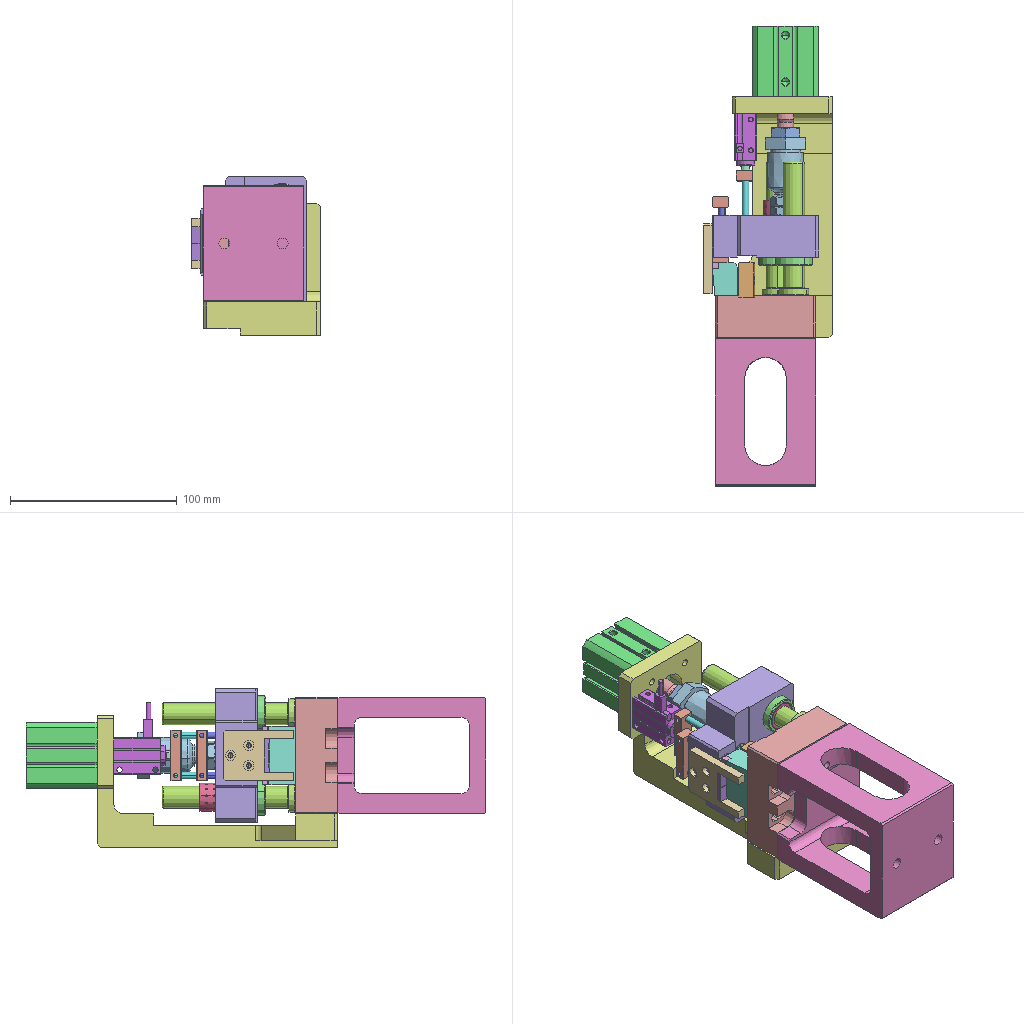Assembly | SolidWorks | 22 different items | 34 placed | box 77 x 276 x 95 mm
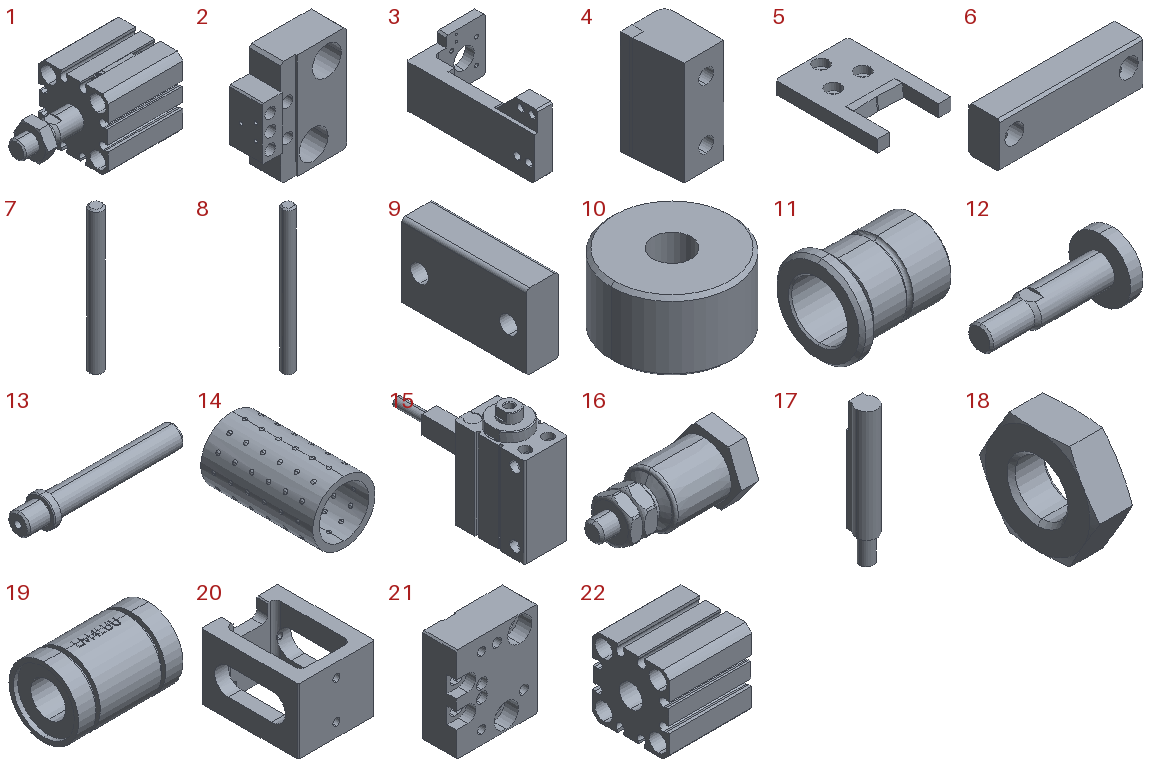Parts list (item | name | quantity | parent item | size | volume | features):
1 | (subassembly) | x1 | - | 75 x 40 x 40 mm | 54113 mm3 | features AEMSimFeature 1
2 | - | x1 | - | 64 x 25 x 80 mm | 85736 mm3 | features ICE 6, Chamfer 2, HoleWzd 2, Extrusion 1
3 | - | x1 | - | 79 x 144 x 70 mm | 147629 mm3 | features ICE 5, Chamfer 3, HoleWzd 3, Fillet 2, Extrusion 1
4 | - | x1 | - | 15 x 20 x 35 mm | 9279 mm3 | features Extrusion 1, Fillet 1, HoleWzd 1, Split 1
5 | - | x1 | - | 30 x 42 x 5 mm | 4509 mm3 | features ICE 3, Chamfer 2, Extrusion 1, Fillet 1, HoleWzd 1
6 | - | x4 | - | 30 x 6.5 x 9.5 mm | 1639 mm3 | features Chamfer 1, Extrusion 1, HoleWzd 1, ICE 1
7 | - | x2 | - | 4 x 4 x 43 mm | 530.221 mm3 | features Chamfer 1, Extrusion 1, ICE 1
8 | - | x2 | - | 4 x 4 x 50 mm | 618.186 mm3 | features Chamfer 1, Extrusion 1, ICE 1
9 | - | x1 | - | 9 x 35 x 21 mm | 5976 mm3 | features HoleWzd 2, Chamfer 1, Extrusion 1, Fillet 1
10 | - | x2 | - | 17.5 x 17.5 x 10 mm | 1853 mm3 | features Chamfer 1, Extrusion 1, ICE 1
11 | - | x2 | - | 30 x 27 x 27 mm | 5060 mm3 | features Chamfer 2, RefAxis 1, RevCut 1, Revolution 1
12 | - | x1 | in 1 | 53.75 x 25 x 25 mm | 7288 mm3 | features RefAxis 6, 3DProfileFeature 2, ICE 1, Revolution 1
13 | - | x2 | - | 93 x 18 x 18 mm | 12586 mm3 | features Chamfer 2, Fillet 1, HoleWzd 1, Revolution 1
14 | - | x2 | - | 17 x 30 x 17 mm | 2413 mm3 | features CirPattern 2, LPattern 2, RefAxis 2, Extrusion 1, ICE 1, Revolution 1
15 | - | x1 | - | 13.5 x 43.2 x 34 mm | 7865 mm3 | features BaseBody 2
16 | - | x1 | - | 54 x 27.472 x 25.615 mm | 13856 mm3 | features ICE 2, Revolution 1
17 | - | x1 | in 1 | 4 x 4.5 x 27 mm | 342.413 mm3 | features ICE 3, RefAxis 3, 3DProfileFeature 1, Extrusion 1, Revolution 1
18 | - | x1 | in 1 | 6 x 19.63 x 17 mm | 1131 mm3 | features RefAxis 3, 3DProfileFeature 1, ICE 1, Revolution 1
19 | - | x4 | - | 12 x 8 x 8 mm | 414.691 mm3 | features Emboss 1, Revolution 1
20 | - | x1 | - | 70 x 89 x 60 mm | 142318 mm3 | features HoleWzd 4, Fillet 2, ICE 2, Chamfer 1, Extrusion 1
21 | - | x1 | - | 60 x 25 x 70 mm | 85234 mm3 | features HoleWzd 7, ICE 3, Chamfer 1, Cut 1, Extrusion 1
22 | - | x1 | in 1 | 42.5 x 40 x 40 mm | 45351 mm3 | features RefAxis 18, 3DProfileFeature 6, HoleWzd 2, RevCut 2, Extrusion 1, LPattern 1
Mates (type | each side: item.copy, entity, surface, feature):
In the top assembly
Concentric | 21.1 face cylinder Cut-Extrude2 | 10.1 face cylinder Boss-Extrude1
Coincident | 21.1 face plane Cut-Extrude2 | 10.1 face plane Boss-Extrude1
Concentric | 21.1 face cylinder Cut-Extrude2 | 10.2 face cylinder Boss-Extrude1
Coincident | 21.1 face plane Cut-Extrude2 | 10.2 face plane Boss-Extrude1
Concentric | 21.1 face cylinder Cut-Extrude1 | 13.1 face cylinder Revolve1
Coincident | 21.1 face plane Boss-Extrude1 | 13.1 face plane Revolve1
Concentric | 21.1 face cylinder Cut-Extrude1 | 13.2 face cylinder Revolve1
Coincident | 21.1 face plane Boss-Extrude1 | 13.2 face plane Revolve1
Width | 21.1 face plane Cut-Extrude1 | 21.1 face plane Cut-Extrude1 | 4.1 face cylinder M6 Tapped Hole1 | 2 times
Coincident | 21.1 face plane Boss-Extrude1 | 4.1 face plane Boss-Extrude1
Coincident | 21.1 face plane Cut-Extrude3 | 9.1 face plane Boss-Extrude1
Concentric | 11.1 face cylinder Revolve1 | 14.1 face cylinder Boss-Extrude1
Coincident | 11.1 face plane Revolve1 | 14.1 face plane Boss-Extrude1
Concentric | 11.2 face cylinder Revolve1 | 14.2 face cylinder Boss-Extrude1
Concentric | 2.1 face cylinder Cut-Extrude1 | 11.2 face cylinder Revolve1
Concentric | 2.1 face cylinder Cut-Extrude1 | 11.1 face cylinder Revolve1
Concentric | 13.2 face cylinder Revolve1 | 14.1 face cylinder Boss-Extrude1
Concentric | 13.1 face cylinder Revolve1 | 14.2 face cylinder Boss-Extrude1
Coincident | 3.1 face plane Boss-Extrude1 | 15.1 face plane Input1
Concentric | 2.1 face cylinder Cut-Extrude7 | 19.1 face cylinder Revolve1
Concentric | 2.1 face cylinder Cut-Extrude7 | 19.2 face cylinder Revolve1
Concentric | 2.1 face cylinder Cut-Extrude7 | 19.3 face cylinder Revolve1
Concentric | 2.1 face cylinder Cut-Extrude7 | 19.4 face cylinder Revolve1
Coincident | 2.1 face plane Cut-Extrude7 | 19.1 face plane Revolve1
Coincident | 2.1 face plane Cut-Extrude7 | 19.2 face plane Revolve1
Coincident | 2.1 face plane Cut-Extrude7 | 19.4 face plane Revolve1
Coincident | 2.1 face plane Cut-Extrude7 | 19.3 face plane Revolve1
Concentric | 6.1 face cylinder Cut-Extrude1 | 7.1 face cylinder Boss-Extrude1
Concentric | 6.1 face cylinder Cut-Extrude1 | 7.2 face cylinder Boss-Extrude1
Concentric | 7.1 face cylinder Boss-Extrude1 | 6.2 face cylinder Cut-Extrude1
Concentric | 7.1 face cylinder Boss-Extrude1 | 19.1 face cylinder Revolve1
Concentric | 19.4 face cylinder Revolve1 | 7.2 face cylinder Boss-Extrude1
Concentric | 6.2 face cylinder Cut-Extrude1 | 7.2 face cylinder Boss-Extrude1
Coincident | 7.1 face plane Boss-Extrude1 | 6.2 face plane Boss-Extrude1
LimitDistanceDim | 2.1 face plane Boss-Extrude1 | 6.2 face plane Boss-Extrude1
LimitDistanceDim | 2.1 face plane Boss-Extrude1 | 16.1 face plane Revolve1
Coincident | 7.1 face plane Boss-Extrude1 | 7.2 edge
Concentric | 21.1 face cylinder M5 Tapped Hole1 | 3.1 face cylinder Hole size per socket head cap screw type1 | 2 times
Coincident | 21.1 face plane Boss-Extrude1 | 3.1 face plane Boss-Extrude1
Concentric | 3.1 face cylinder M3 Tapped Hole1 | 15.1 face cylinder Input1 | 2 times
Concentric | 2.1 face cylinder M8 Tapped Hole1 | 16.1 face cylinder Revolve1
Concentric | 21.1 face cylinder Hole size per socket head cap screw type2 | 9.1 face cylinder M4 Tapped Hole1
Coincident | 21.1 face plane Boss-Extrude1 | 20.1 face plane Boss-Extrude1
Coincident | 2.1 face plane Cut-Extrude12 | 11.1 face plane Revolve1
Coincident | 2.1 face plane Cut-Extrude12 | 11.2 face plane Revolve1
Coincident | 6.1 face plane Boss-Extrude1 | 7.1 face plane Boss-Extrude1
Concentric | 6.3 face cylinder Cut-Extrude1 | 8.1 face cylinder Boss-Extrude1
Coincident | 6.3 face plane Boss-Extrude1 | 8.1 face plane Boss-Extrude1
Concentric | 6.3 face cylinder Cut-Extrude1 | 8.2 face cylinder Boss-Extrude1
Coincident | 6.3 face plane Boss-Extrude1 | 8.2 face plane Boss-Extrude1
Concentric | 19.2 face cylinder Revolve1 | 8.2 face cylinder Boss-Extrude1
Concentric | 19.3 face cylinder Revolve1 | 8.1 face cylinder Boss-Extrude1
Concentric | 6.4 face cylinder Cut-Extrude1 | 8.2 face cylinder Boss-Extrude1
Concentric | 6.4 face cylinder Cut-Extrude1 | 8.1 face cylinder Boss-Extrude1
Coincident | 6.4 face plane Boss-Extrude1 | 8.1 face plane Boss-Extrude1
Coincident | 2.1 face plane Boss-Extrude1 | 5.1 face plane Boss-Extrude1
Concentric | 2.1 face cylinder M3 Tapped Hole1 | 5.1 face cylinder CBORE for M3 Hex Head Bolt1 | 2 times
Concentric | 21.1 face cylinder Hole size per socket head cap screw type3 | 20.1 face cylinder M6 Tapped Hole1 | 2 times
Coincident | 3.1 face plane Boss-Extrude1 | 22.1 face plane Boss-Extrude1
Concentric | 3.1 face cylinder M5 Tapped Hole1 | 22.1 face cylinder LPattern1
Concentric | 3.1 face cylinder Cut-Extrude2 | 12.1 face cylinder Revolve1
Coincident | 16.1 face plane Revolve1 | 18.1 face plane Revolve1
In subassembly 1
Concentric | 22.2 face cylinder Cut-Revolve2 | 12.2 face cylinder Revolve1
DistanceDim | 22.2 face plane Cut-Revolve2 | 12.2 face plane Revolve1
PlanarAngleDim | 12.2 plane | 1.1 plane
PlanarAngleDim | 18.2 plane | 1.1 plane
DistanceDim | 17.1 face plane Boss-Extrude1 | 22.2 face plane Boss-Extrude1
Concentric | 22.2 face cylinder Boss-Extrude1 | 17.1 face cylinder Boss-Extrude1
PlanarAngleDim | 22.2 face plane Boss-Extrude1 | 17.1 face plane Boss-Extrude1
Concentric | 12.2 face cylinder Revolve1 | 18.2 face cylinder Revolve1
DistanceDim | 12.2 face plane Revolve1 | 18.2 face plane Revolve1